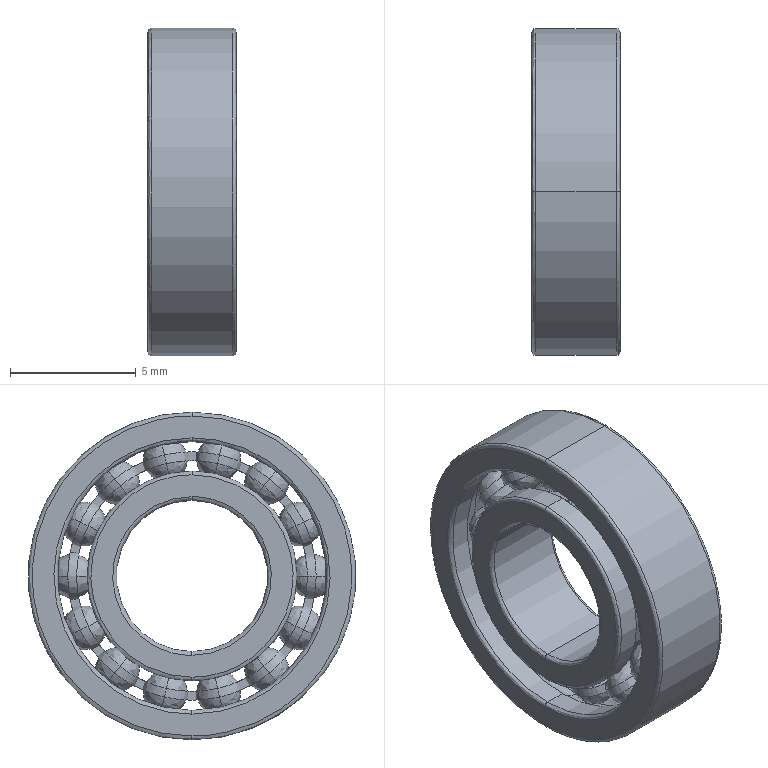Part | SolidWorks | features BaseBody 16 | 16 solids | 179 faces | box 3.5 x 13 x 13 mm | volume 272.002 mm3 | spline 81 | cylinder 66 | plane 32 | commonest cylinder face diameters 9.15 x27 9.85 x27 8.333 x4 10.667 x4 6 x2 13 x2